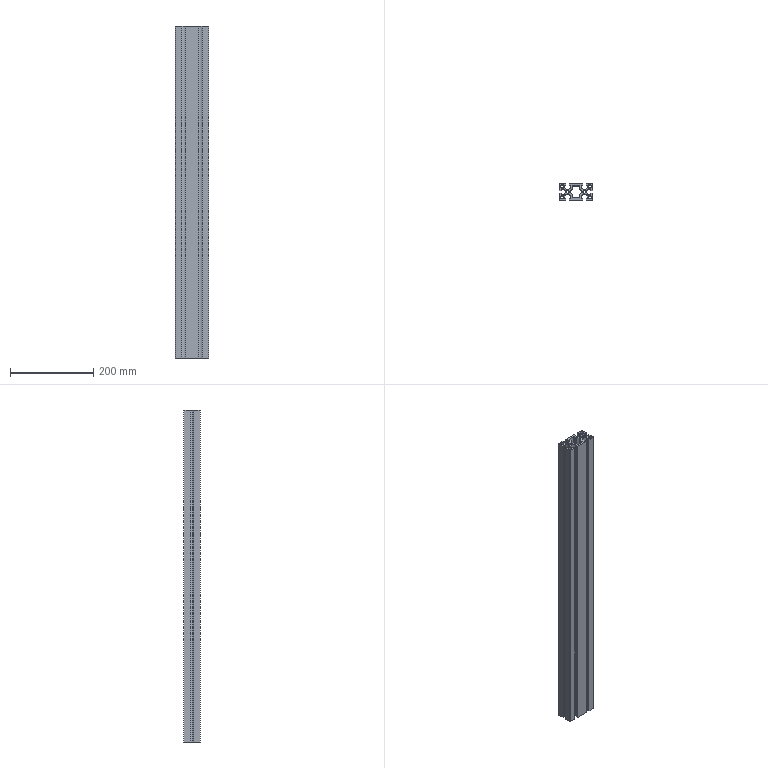Part | STEP file | 40x80 aluminium profile (L=800) | 1 solid | 87 faces | box 80 x 40 x 800 mm | volume 1067295 mm3 | plane 60 | cylinder 27 | commonest cylinder face diameters 8 x8 17.549 x7 1 x4 4 x4 6.8 x4